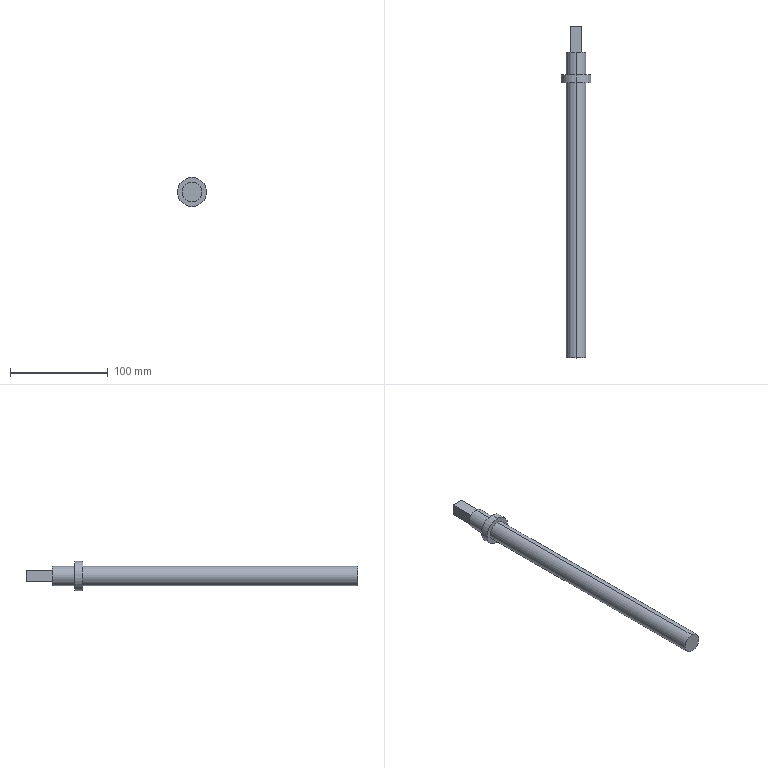Part | SolidWorks | features Cut 1, Extrusion 1, ICE 1 | 1 solid | 15 faces | box 30 x 340 x 30 mm | volume 105361 mm3 | plane 9 | cylinder 6 | commonest cylinder face diameters 20 x4 30 x2
STEP:
#1=CARTESIAN_POINT('',(0.,282.,10.));
#2=VERTEX_POINT('',#1);
#3=CARTESIAN_POINT('',(0.,282.,-10.));
#4=VERTEX_POINT('',#3);
#5=CARTESIAN_POINT('',(0.,282.,0.));
#6=DIRECTION('',(0.,1.,0.));
#7=DIRECTION('',(0.,0.,1.));
#8=AXIS2_PLACEMENT_3D('',#5,#6,#7);
#9=CIRCLE('',#8,10.);
#10=EDGE_CURVE('',#2,#4,#9,.T.);
#11=ORIENTED_EDGE('',*,*,#10,.F.);
#12=CARTESIAN_POINT('',(0.,0.,10.));
#13=VERTEX_POINT('',#12);
#14=CARTESIAN_POINT('',(0.,340.,10.));
#15=DIRECTION('',(0.,-1.,0.));
#16=VECTOR('',#15,1000.);
#17=LINE('',#14,#16);
#18=EDGE_CURVE('',#2,#13,#17,.T.);
#19=ORIENTED_EDGE('',*,*,#18,.T.);
#20=CARTESIAN_POINT('',(0.,0.,-10.));
#21=VERTEX_POINT('',#20);
#22=CARTESIAN_POINT('',(0.,0.,0.));
#23=DIRECTION('',(0.,1.,0.));
#24=DIRECTION('',(0.,0.,1.));
#25=AXIS2_PLACEMENT_3D('',#22,#23,#24);
#26=CIRCLE('',#25,10.);
#27=EDGE_CURVE('',#13,#21,#26,.T.);
#28=ORIENTED_EDGE('',*,*,#27,.T.);
#29=CARTESIAN_POINT('',(0.,340.,-10.));
#30=DIRECTION('',(0.,-1.,0.));
#31=VECTOR('',#30,1000.);
#32=LINE('',#29,#31);
#33=EDGE_CURVE('',#4,#21,#32,.T.);
#34=ORIENTED_EDGE('',*,*,#33,.F.);
#35=EDGE_LOOP('',(#11,#19,#28,#34));
#36=FACE_OUTER_BOUND('',#35,.T.);
#37=CARTESIAN_POINT('',(0.,340.,0.));
#38=DIRECTION('',(0.,-1.,0.));
#39=DIRECTION('',(0.,0.,-1.));
#40=AXIS2_PLACEMENT_3D('',#37,#38,#39);
#41=CYLINDRICAL_SURFACE('',#40,10.);
#42=ADVANCED_FACE('',(#36),#41,.T.);
#43=CARTESIAN_POINT('',(0.,290.,15.));
#44=VERTEX_POINT('',#43);
#45=CARTESIAN_POINT('',(0.,290.,-15.));
#46=VERTEX_POINT('',#45);
#47=CARTESIAN_POINT('',(0.,290.,0.));
#48=DIRECTION('',(0.,1.,0.));
#49=DIRECTION('',(0.,0.,1.));
#50=AXIS2_PLACEMENT_3D('',#47,#48,#49);
#51=CIRCLE('',#50,15.);
#52=EDGE_CURVE('',#44,#46,#51,.T.);
#53=ORIENTED_EDGE('',*,*,#52,.F.);
#54=CARTESIAN_POINT('',(0.,282.,15.));
#55=VERTEX_POINT('',#54);
#56=CARTESIAN_POINT('',(0.,290.,15.));
#57=DIRECTION('',(0.,-1.,0.));
#58=VECTOR('',#57,1000.);
#59=LINE('',#56,#58);
#60=EDGE_CURVE('',#44,#55,#59,.T.);
#61=ORIENTED_EDGE('',*,*,#60,.T.);
#62=CARTESIAN_POINT('',(0.,282.,-15.));
#63=VERTEX_POINT('',#62);
#64=CARTESIAN_POINT('',(0.,282.,0.));
#65=DIRECTION('',(0.,1.,0.));
#66=DIRECTION('',(0.,0.,1.));
#67=AXIS2_PLACEMENT_3D('',#64,#65,#66);
#68=CIRCLE('',#67,15.);
#69=EDGE_CURVE('',#55,#63,#68,.T.);
#70=ORIENTED_EDGE('',*,*,#69,.T.);
#71=CARTESIAN_POINT('',(0.,290.,-15.));
#72=DIRECTION('',(0.,-1.,0.));
#73=VECTOR('',#72,1000.);
#74=LINE('',#71,#73);
#75=EDGE_CURVE('',#46,#63,#74,.T.);
#76=ORIENTED_EDGE('',*,*,#75,.F.);
#77=EDGE_LOOP('',(#53,#61,#70,#76));
#78=FACE_OUTER_BOUND('',#77,.T.);
#79=CARTESIAN_POINT('',(0.,290.,0.));
#80=DIRECTION('',(0.,-1.,0.));
#81=DIRECTION('',(0.,0.,-1.));
#82=AXIS2_PLACEMENT_3D('',#79,#80,#81);
#83=CYLINDRICAL_SURFACE('',#82,15.);
#84=ADVANCED_FACE('',(#78),#83,.T.);
#85=CARTESIAN_POINT('',(0.,313.,10.));
#86=VERTEX_POINT('',#85);
#87=CARTESIAN_POINT('',(0.,313.,-10.));
#88=VERTEX_POINT('',#87);
#89=CARTESIAN_POINT('',(0.,313.,0.));
#90=DIRECTION('',(0.,1.,0.));
#91=DIRECTION('',(0.,0.,1.));
#92=AXIS2_PLACEMENT_3D('',#89,#90,#91);
#93=CIRCLE('',#92,10.);
#94=EDGE_CURVE('',#86,#88,#93,.T.);
#95=ORIENTED_EDGE('',*,*,#94,.F.);
#96=CARTESIAN_POINT('',(0.,290.,10.));
#97=VERTEX_POINT('',#96);
#98=CARTESIAN_POINT('',(0.,340.,10.));
#99=DIRECTION('',(0.,-1.,0.));
#100=VECTOR('',#99,1000.);
#101=LINE('',#98,#100);
#102=EDGE_CURVE('',#86,#97,#101,.T.);
#103=ORIENTED_EDGE('',*,*,#102,.T.);
#104=CARTESIAN_POINT('',(0.,290.,-10.));
#105=VERTEX_POINT('',#104);
#106=CARTESIAN_POINT('',(0.,290.,0.));
#107=DIRECTION('',(0.,1.,0.));
#108=DIRECTION('',(0.,0.,1.));
#109=AXIS2_PLACEMENT_3D('',#106,#107,#108);
#110=CIRCLE('',#109,10.);
#111=EDGE_CURVE('',#97,#105,#110,.T.);
#112=ORIENTED_EDGE('',*,*,#111,.T.);
#113=CARTESIAN_POINT('',(0.,340.,-10.));
#114=DIRECTION('',(0.,-1.,0.));
#115=VECTOR('',#114,1000.);
#116=LINE('',#113,#115);
#117=EDGE_CURVE('',#88,#105,#116,.T.);
#118=ORIENTED_EDGE('',*,*,#117,.F.);
#119=EDGE_LOOP('',(#95,#103,#112,#118));
#120=FACE_OUTER_BOUND('',#119,.T.);
#121=CARTESIAN_POINT('',(0.,340.,0.));
#122=DIRECTION('',(0.,-1.,0.));
#123=DIRECTION('',(0.,0.,-1.));
#124=AXIS2_PLACEMENT_3D('',#121,#122,#123);
#125=CYLINDRICAL_SURFACE('',#124,10.);
#126=ADVANCED_FACE('',(#120),#125,.T.);
#127=ORIENTED_EDGE('',*,*,#102,.F.);
#128=CARTESIAN_POINT('',(0.,313.,0.));
#129=DIRECTION('',(0.,1.,0.));
#130=DIRECTION('',(0.,0.,1.));
#131=AXIS2_PLACEMENT_3D('',#128,#129,#130);
#132=CIRCLE('',#131,10.);
#133=EDGE_CURVE('',#88,#86,#132,.T.);
#134=ORIENTED_EDGE('',*,*,#133,.F.);
#135=ORIENTED_EDGE('',*,*,#117,.T.);
#136=CARTESIAN_POINT('',(0.,290.,0.));
#137=DIRECTION('',(0.,1.,0.));
#138=DIRECTION('',(0.,0.,1.));
#139=AXIS2_PLACEMENT_3D('',#136,#137,#138);
#140=CIRCLE('',#139,10.);
#141=EDGE_CURVE('',#105,#97,#140,.T.);
#142=ORIENTED_EDGE('',*,*,#141,.T.);
#143=EDGE_LOOP('',(#127,#134,#135,#142));
#144=FACE_OUTER_BOUND('',#143,.T.);
#145=CARTESIAN_POINT('',(0.,340.,0.));
#146=DIRECTION('',(0.,-1.,0.));
#147=DIRECTION('',(0.,0.,-1.));
#148=AXIS2_PLACEMENT_3D('',#145,#146,#147);
#149=CYLINDRICAL_SURFACE('',#148,10.);
#150=ADVANCED_FACE('',(#144),#149,.T.);
#151=CARTESIAN_POINT('',(-6.,313.,6.));
#152=VERTEX_POINT('',#151);
#153=CARTESIAN_POINT('',(6.,313.,6.));
#154=VERTEX_POINT('',#153);
#155=CARTESIAN_POINT('',(-6.,313.,6.));
#156=DIRECTION('',(1.,0.,0.));
#157=VECTOR('',#156,1000.);
#158=LINE('',#155,#157);
#159=EDGE_CURVE('',#152,#154,#158,.T.);
#160=ORIENTED_EDGE('',*,*,#159,.F.);
#161=CARTESIAN_POINT('',(-6.,313.,-6.));
#162=VERTEX_POINT('',#161);
#163=CARTESIAN_POINT('',(-6.,313.,-6.));
#164=DIRECTION('',(0.,0.,1.));
#165=VECTOR('',#164,1000.);
#166=LINE('',#163,#165);
#167=EDGE_CURVE('',#162,#152,#166,.T.);
#168=ORIENTED_EDGE('',*,*,#167,.F.);
#169=CARTESIAN_POINT('',(6.,313.,-6.));
#170=VERTEX_POINT('',#169);
#171=CARTESIAN_POINT('',(-6.,313.,-6.));
#172=DIRECTION('',(-1.,0.,0.));
#173=VECTOR('',#172,1000.);
#174=LINE('',#171,#173);
#175=EDGE_CURVE('',#170,#162,#174,.T.);
#176=ORIENTED_EDGE('',*,*,#175,.F.);
#177=CARTESIAN_POINT('',(6.,313.,-6.));
#178=DIRECTION('',(0.,0.,-1.));
#179=VECTOR('',#178,1000.);
#180=LINE('',#177,#179);
#181=EDGE_CURVE('',#154,#170,#180,.T.);
#182=ORIENTED_EDGE('',*,*,#181,.F.);
#183=EDGE_LOOP('',(#160,#168,#176,#182));
#184=FACE_BOUND('',#183,.T.);
#185=ORIENTED_EDGE('',*,*,#133,.T.);
#186=ORIENTED_EDGE('',*,*,#94,.T.);
#187=EDGE_LOOP('',(#185,#186));
#188=FACE_OUTER_BOUND('',#187,.T.);
#189=CARTESIAN_POINT('',(0.,313.,0.));
#190=DIRECTION('',(0.,1.,0.));
#191=DIRECTION('',(0.,0.,1.));
#192=AXIS2_PLACEMENT_3D('',#189,#190,#191);
#193=PLANE('',#192);
#194=ADVANCED_FACE('',(#184,#188),#193,.T.);
#195=CARTESIAN_POINT('',(6.,340.,6.));
#196=VERTEX_POINT('',#195);
#197=CARTESIAN_POINT('',(6.,340.,-6.));
#198=VERTEX_POINT('',#197);
#199=CARTESIAN_POINT('',(6.,340.,-6.));
#200=DIRECTION('',(0.,0.,-1.));
#201=VECTOR('',#200,1000.);
#202=LINE('',#199,#201);
#203=EDGE_CURVE('',#196,#198,#202,.T.);
#204=ORIENTED_EDGE('',*,*,#203,.F.);
#205=CARTESIAN_POINT('',(6.,313.,6.));
#206=DIRECTION('',(0.,1.,0.));
#207=VECTOR('',#206,1000.);
#208=LINE('',#205,#207);
#209=EDGE_CURVE('',#154,#196,#208,.T.);
#210=ORIENTED_EDGE('',*,*,#209,.F.);
#211=ORIENTED_EDGE('',*,*,#181,.T.);
#212=CARTESIAN_POINT('',(6.,313.,-6.));
#213=DIRECTION('',(0.,1.,0.));
#214=VECTOR('',#213,1000.);
#215=LINE('',#212,#214);
#216=EDGE_CURVE('',#170,#198,#215,.T.);
#217=ORIENTED_EDGE('',*,*,#216,.T.);
#218=EDGE_LOOP('',(#204,#210,#211,#217));
#219=FACE_OUTER_BOUND('',#218,.T.);
#220=CARTESIAN_POINT('',(6.,313.,-6.));
#221=DIRECTION('',(1.,0.,0.));
#222=DIRECTION('',(0.,0.,-1.));
#223=AXIS2_PLACEMENT_3D('',#220,#221,#222);
#224=PLANE('',#223);
#225=ADVANCED_FACE('',(#219),#224,.T.);
#226=CARTESIAN_POINT('',(-6.,340.,6.));
#227=VERTEX_POINT('',#226);
#228=CARTESIAN_POINT('',(-6.,340.,6.));
#229=DIRECTION('',(1.,0.,0.));
#230=VECTOR('',#229,1000.);
#231=LINE('',#228,#230);
#232=EDGE_CURVE('',#227,#196,#231,.T.);
#233=ORIENTED_EDGE('',*,*,#232,.F.);
#234=CARTESIAN_POINT('',(-6.,313.,6.));
#235=DIRECTION('',(0.,1.,0.));
#236=VECTOR('',#235,1000.);
#237=LINE('',#234,#236);
#238=EDGE_CURVE('',#152,#227,#237,.T.);
#239=ORIENTED_EDGE('',*,*,#238,.F.);
#240=ORIENTED_EDGE('',*,*,#159,.T.);
#241=ORIENTED_EDGE('',*,*,#209,.T.);
#242=EDGE_LOOP('',(#233,#239,#240,#241));
#243=FACE_OUTER_BOUND('',#242,.T.);
#244=CARTESIAN_POINT('',(-6.,313.,6.));
#245=DIRECTION('',(0.,0.,1.));
#246=DIRECTION('',(1.,0.,0.));
#247=AXIS2_PLACEMENT_3D('',#244,#245,#246);
#248=PLANE('',#247);
#249=ADVANCED_FACE('',(#243),#248,.T.);
#250=CARTESIAN_POINT('',(-6.,340.,-6.));
#251=VERTEX_POINT('',#250);
#252=CARTESIAN_POINT('',(-6.,340.,-6.));
#253=DIRECTION('',(0.,0.,1.));
#254=VECTOR('',#253,1000.);
#255=LINE('',#252,#254);
#256=EDGE_CURVE('',#251,#227,#255,.T.);
#257=ORIENTED_EDGE('',*,*,#256,.F.);
#258=CARTESIAN_POINT('',(-6.,313.,-6.));
#259=DIRECTION('',(0.,1.,0.));
#260=VECTOR('',#259,1000.);
#261=LINE('',#258,#260);
#262=EDGE_CURVE('',#162,#251,#261,.T.);
#263=ORIENTED_EDGE('',*,*,#262,.F.);
#264=ORIENTED_EDGE('',*,*,#167,.T.);
#265=ORIENTED_EDGE('',*,*,#238,.T.);
#266=EDGE_LOOP('',(#257,#263,#264,#265));
#267=FACE_OUTER_BOUND('',#266,.T.);
#268=CARTESIAN_POINT('',(-6.,313.,-6.));
#269=DIRECTION('',(-1.,0.,0.));
#270=DIRECTION('',(0.,0.,1.));
#271=AXIS2_PLACEMENT_3D('',#268,#269,#270);
#272=PLANE('',#271);
#273=ADVANCED_FACE('',(#267),#272,.T.);
#274=CARTESIAN_POINT('',(-6.,340.,-6.));
#275=DIRECTION('',(-1.,0.,0.));
#276=VECTOR('',#275,1000.);
#277=LINE('',#274,#276);
#278=EDGE_CURVE('',#198,#251,#277,.T.);
#279=ORIENTED_EDGE('',*,*,#278,.F.);
#280=ORIENTED_EDGE('',*,*,#216,.F.);
#281=ORIENTED_EDGE('',*,*,#175,.T.);
#282=ORIENTED_EDGE('',*,*,#262,.T.);
#283=EDGE_LOOP('',(#279,#280,#281,#282));
#284=FACE_OUTER_BOUND('',#283,.T.);
#285=CARTESIAN_POINT('',(-6.,313.,-6.));
#286=DIRECTION('',(0.,0.,-1.));
#287=DIRECTION('',(-1.,0.,0.));
#288=AXIS2_PLACEMENT_3D('',#285,#286,#287);
#289=PLANE('',#288);
#290=ADVANCED_FACE('',(#284),#289,.T.);
#291=ORIENTED_EDGE('',*,*,#232,.T.);
#292=ORIENTED_EDGE('',*,*,#203,.T.);
#293=ORIENTED_EDGE('',*,*,#278,.T.);
#294=ORIENTED_EDGE('',*,*,#256,.T.);
#295=EDGE_LOOP('',(#291,#292,#293,#294));
#296=FACE_OUTER_BOUND('',#295,.T.);
#297=CARTESIAN_POINT('',(0.,340.,0.));
#298=DIRECTION('',(0.,1.,0.));
#299=DIRECTION('',(0.,0.,1.));
#300=AXIS2_PLACEMENT_3D('',#297,#298,#299);
#301=PLANE('',#300);
#302=ADVANCED_FACE('',(#296),#301,.T.);
#303=ORIENTED_EDGE('',*,*,#60,.F.);
#304=CARTESIAN_POINT('',(0.,290.,0.));
#305=DIRECTION('',(0.,1.,0.));
#306=DIRECTION('',(0.,0.,1.));
#307=AXIS2_PLACEMENT_3D('',#304,#305,#306);
#308=CIRCLE('',#307,15.);
#309=EDGE_CURVE('',#46,#44,#308,.T.);
#310=ORIENTED_EDGE('',*,*,#309,.F.);
#311=ORIENTED_EDGE('',*,*,#75,.T.);
#312=CARTESIAN_POINT('',(0.,282.,0.));
#313=DIRECTION('',(0.,1.,0.));
#314=DIRECTION('',(0.,0.,1.));
#315=AXIS2_PLACEMENT_3D('',#312,#313,#314);
#316=CIRCLE('',#315,15.);
#317=EDGE_CURVE('',#63,#55,#316,.T.);
#318=ORIENTED_EDGE('',*,*,#317,.T.);
#319=EDGE_LOOP('',(#303,#310,#311,#318));
#320=FACE_OUTER_BOUND('',#319,.T.);
#321=CARTESIAN_POINT('',(0.,290.,0.));
#322=DIRECTION('',(0.,-1.,0.));
#323=DIRECTION('',(0.,0.,-1.));
#324=AXIS2_PLACEMENT_3D('',#321,#322,#323);
#325=CYLINDRICAL_SURFACE('',#324,15.);
#326=ADVANCED_FACE('',(#320),#325,.T.);
#327=ORIENTED_EDGE('',*,*,#141,.F.);
#328=ORIENTED_EDGE('',*,*,#111,.F.);
#329=EDGE_LOOP('',(#327,#328));
#330=FACE_BOUND('',#329,.T.);
#331=ORIENTED_EDGE('',*,*,#309,.T.);
#332=ORIENTED_EDGE('',*,*,#52,.T.);
#333=EDGE_LOOP('',(#331,#332));
#334=FACE_OUTER_BOUND('',#333,.T.);
#335=CARTESIAN_POINT('',(0.,290.,0.));
#336=DIRECTION('',(0.,1.,0.));
#337=DIRECTION('',(0.,0.,1.));
#338=AXIS2_PLACEMENT_3D('',#335,#336,#337);
#339=PLANE('',#338);
#340=ADVANCED_FACE('',(#330,#334),#339,.T.);
#341=CARTESIAN_POINT('',(0.,282.,0.));
#342=DIRECTION('',(0.,1.,0.));
#343=DIRECTION('',(0.,0.,1.));
#344=AXIS2_PLACEMENT_3D('',#341,#342,#343);
#345=CIRCLE('',#344,10.);
#346=EDGE_CURVE('',#4,#2,#345,.T.);
#347=ORIENTED_EDGE('',*,*,#346,.T.);
#348=ORIENTED_EDGE('',*,*,#10,.T.);
#349=EDGE_LOOP('',(#347,#348));
#350=FACE_BOUND('',#349,.T.);
#351=ORIENTED_EDGE('',*,*,#317,.F.);
#352=ORIENTED_EDGE('',*,*,#69,.F.);
#353=EDGE_LOOP('',(#351,#352));
#354=FACE_OUTER_BOUND('',#353,.T.);
#355=CARTESIAN_POINT('',(0.,282.,0.));
#356=DIRECTION('',(0.,1.,0.));
#357=DIRECTION('',(0.,0.,1.));
#358=AXIS2_PLACEMENT_3D('',#355,#356,#357);
#359=PLANE('',#358);
#360=ADVANCED_FACE('',(#350,#354),#359,.F.);
#361=CARTESIAN_POINT('',(0.,0.,0.));
#362=DIRECTION('',(0.,1.,0.));
#363=DIRECTION('',(0.,0.,1.));
#364=AXIS2_PLACEMENT_3D('',#361,#362,#363);
#365=CIRCLE('',#364,10.);
#366=EDGE_CURVE('',#21,#13,#365,.T.);
#367=ORIENTED_EDGE('',*,*,#366,.F.);
#368=ORIENTED_EDGE('',*,*,#27,.F.);
#369=EDGE_LOOP('',(#367,#368));
#370=FACE_OUTER_BOUND('',#369,.T.);
#371=CARTESIAN_POINT('',(0.,0.,0.));
#372=DIRECTION('',(0.,1.,0.));
#373=DIRECTION('',(0.,0.,1.));
#374=AXIS2_PLACEMENT_3D('',#371,#372,#373);
#375=PLANE('',#374);
#376=ADVANCED_FACE('',(#370),#375,.F.);
#377=ORIENTED_EDGE('',*,*,#18,.F.);
#378=ORIENTED_EDGE('',*,*,#346,.F.);
#379=ORIENTED_EDGE('',*,*,#33,.T.);
#380=ORIENTED_EDGE('',*,*,#366,.T.);
#381=EDGE_LOOP('',(#377,#378,#379,#380));
#382=FACE_OUTER_BOUND('',#381,.T.);
#383=CARTESIAN_POINT('',(0.,340.,0.));
#384=DIRECTION('',(0.,-1.,0.));
#385=DIRECTION('',(0.,0.,-1.));
#386=AXIS2_PLACEMENT_3D('',#383,#384,#385);
#387=CYLINDRICAL_SURFACE('',#386,10.);
#388=ADVANCED_FACE('',(#382),#387,.T.);
#389=CLOSED_SHELL('',(#42,#84,#126,#150,#194,#225,#249,#273,#290,#302,#326,#340,#360,#376,#388));
#390=MANIFOLD_SOLID_BREP('',#389);
#391=CARTESIAN_POINT('',(0.,0.,0.));
#392=DIRECTION('',(0.,0.,1.));
#393=DIRECTION('',(1.,0.,0.));
#394=AXIS2_PLACEMENT_3D('',#391,#392,#393);
#395=(LENGTH_UNIT()NAMED_UNIT(*)SI_UNIT(.MILLI.,.METRE.));
#396=UNCERTAINTY_MEASURE_WITH_UNIT(LENGTH_MEASURE(0.00001),#395,'','');
#397=(NAMED_UNIT(*)PLANE_ANGLE_UNIT()SI_UNIT($,.RADIAN.));
#398=(NAMED_UNIT(*)SI_UNIT($,.STERADIAN.)SOLID_ANGLE_UNIT());
#399=(GEOMETRIC_REPRESENTATION_CONTEXT(3)GLOBAL_UNCERTAINTY_ASSIGNED_CONTEXT((#396))GLOBAL_UNIT_ASSIGNED_CONTEXT((#395,#397,#398))REPRESENTATION_CONTEXT('',''));
#400=ADVANCED_BREP_SHAPE_REPRESENTATION('',(#390,#394),#399);